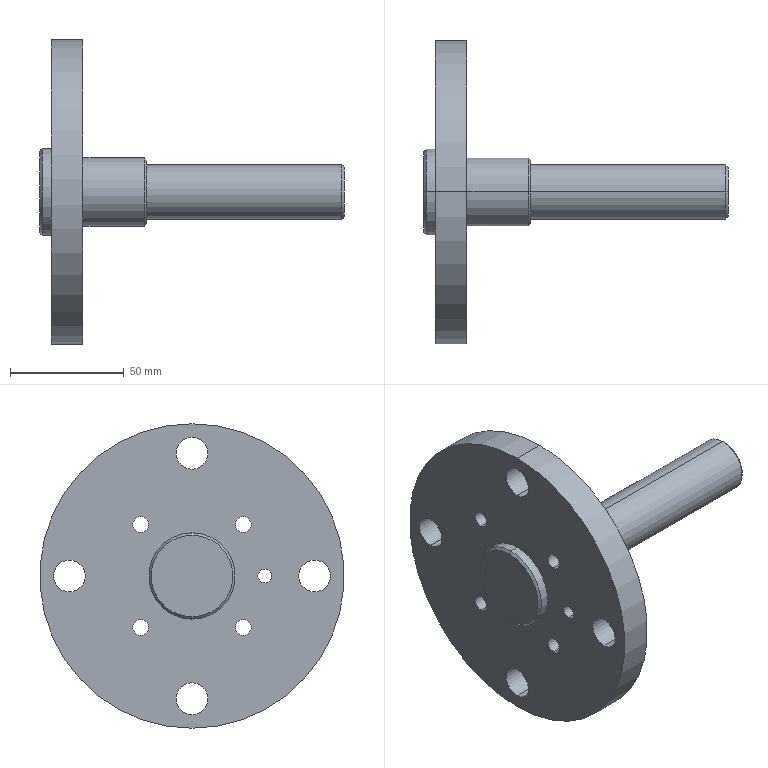Part | SolidWorks | features ICE 8, Chamfer 2, CirPattern 2, Revolution 1 | 1 solid | 49 faces | box 134 x 134 x 134 mm | volume 249153 mm3 | cylinder 34 | plane 9 | cone 6 | commonest cylinder face diameters 7 x8 12 x8 14 x8 6 x2 24 x2 30 x2
STEP:
#1=CARTESIAN_POINT('',(92.,0.,47.));
#2=VERTEX_POINT('',#1);
#3=CARTESIAN_POINT('',(92.,0.,61.));
#4=VERTEX_POINT('',#3);
#5=CARTESIAN_POINT('',(92.,0.,54.));
#6=DIRECTION('',(-1.,0.,0.));
#7=DIRECTION('',(0.,0.,1.));
#8=AXIS2_PLACEMENT_3D('',#5,#6,#7);
#9=CIRCLE('',#8,7.);
#10=EDGE_CURVE('',#2,#4,#9,.T.);
#11=ORIENTED_EDGE('',*,*,#10,.F.);
#12=CARTESIAN_POINT('',(78.,0.,47.));
#13=VERTEX_POINT('',#12);
#14=CARTESIAN_POINT('',(119.,0.,47.));
#15=DIRECTION('',(-1.,0.,0.));
#16=VECTOR('',#15,1000.);
#17=LINE('',#14,#16);
#18=EDGE_CURVE('',#2,#13,#17,.T.);
#19=ORIENTED_EDGE('',*,*,#18,.T.);
#20=CARTESIAN_POINT('',(78.,0.,61.));
#21=VERTEX_POINT('',#20);
#22=CARTESIAN_POINT('',(78.,0.,54.));
#23=DIRECTION('',(-1.,0.,0.));
#24=DIRECTION('',(0.,1.,0.));
#25=AXIS2_PLACEMENT_3D('',#22,#23,#24);
#26=CIRCLE('',#25,7.);
#27=EDGE_CURVE('',#13,#21,#26,.T.);
#28=ORIENTED_EDGE('',*,*,#27,.T.);
#29=CARTESIAN_POINT('',(119.,0.,61.));
#30=DIRECTION('',(-1.,0.,0.));
#31=VECTOR('',#30,1000.);
#32=LINE('',#29,#31);
#33=EDGE_CURVE('',#4,#21,#32,.T.);
#34=ORIENTED_EDGE('',*,*,#33,.F.);
#35=EDGE_LOOP('',(#11,#19,#28,#34));
#36=FACE_OUTER_BOUND('',#35,.T.);
#37=CARTESIAN_POINT('',(119.,0.,54.));
#38=DIRECTION('',(-1.,0.,0.));
#39=DIRECTION('',(0.,0.,1.));
#40=AXIS2_PLACEMENT_3D('',#37,#38,#39);
#41=CYLINDRICAL_SURFACE('',#40,7.);
#42=ADVANCED_FACE('',(#36),#41,.F.);
#43=CARTESIAN_POINT('',(92.,54.,-7.));
#44=VERTEX_POINT('',#43);
#45=CARTESIAN_POINT('',(92.,54.,7.));
#46=VERTEX_POINT('',#45);
#47=CARTESIAN_POINT('',(92.,54.,0.));
#48=DIRECTION('',(-1.,0.,0.));
#49=DIRECTION('',(0.,0.,1.));
#50=AXIS2_PLACEMENT_3D('',#47,#48,#49);
#51=CIRCLE('',#50,7.);
#52=EDGE_CURVE('',#44,#46,#51,.T.);
#53=ORIENTED_EDGE('',*,*,#52,.F.);
#54=CARTESIAN_POINT('',(78.,54.,-7.));
#55=VERTEX_POINT('',#54);
#56=CARTESIAN_POINT('',(119.,54.,-7.));
#57=DIRECTION('',(-1.,0.,0.));
#58=VECTOR('',#57,1000.);
#59=LINE('',#56,#58);
#60=EDGE_CURVE('',#44,#55,#59,.T.);
#61=ORIENTED_EDGE('',*,*,#60,.T.);
#62=CARTESIAN_POINT('',(78.,54.,7.));
#63=VERTEX_POINT('',#62);
#64=CARTESIAN_POINT('',(78.,54.,0.));
#65=DIRECTION('',(-1.,0.,0.));
#66=DIRECTION('',(0.,0.,-1.));
#67=AXIS2_PLACEMENT_3D('',#64,#65,#66);
#68=CIRCLE('',#67,7.);
#69=EDGE_CURVE('',#55,#63,#68,.T.);
#70=ORIENTED_EDGE('',*,*,#69,.T.);
#71=CARTESIAN_POINT('',(119.,54.,7.));
#72=DIRECTION('',(-1.,0.,0.));
#73=VECTOR('',#72,1000.);
#74=LINE('',#71,#73);
#75=EDGE_CURVE('',#46,#63,#74,.T.);
#76=ORIENTED_EDGE('',*,*,#75,.F.);
#77=EDGE_LOOP('',(#53,#61,#70,#76));
#78=FACE_OUTER_BOUND('',#77,.T.);
#79=CARTESIAN_POINT('',(119.,54.,0.));
#80=DIRECTION('',(-1.,0.,0.));
#81=DIRECTION('',(0.,0.,1.));
#82=AXIS2_PLACEMENT_3D('',#79,#80,#81);
#83=CYLINDRICAL_SURFACE('',#82,7.);
#84=ADVANCED_FACE('',(#78),#83,.F.);
#85=CARTESIAN_POINT('',(92.,0.,-61.));
#86=VERTEX_POINT('',#85);
#87=CARTESIAN_POINT('',(92.,0.,-47.));
#88=VERTEX_POINT('',#87);
#89=CARTESIAN_POINT('',(92.,0.,-54.));
#90=DIRECTION('',(-1.,0.,0.));
#91=DIRECTION('',(0.,0.,1.));
#92=AXIS2_PLACEMENT_3D('',#89,#90,#91);
#93=CIRCLE('',#92,7.);
#94=EDGE_CURVE('',#86,#88,#93,.T.);
#95=ORIENTED_EDGE('',*,*,#94,.F.);
#96=CARTESIAN_POINT('',(78.,0.,-61.));
#97=VERTEX_POINT('',#96);
#98=CARTESIAN_POINT('',(119.,0.,-61.));
#99=DIRECTION('',(-1.,0.,0.));
#100=VECTOR('',#99,1000.);
#101=LINE('',#98,#100);
#102=EDGE_CURVE('',#86,#97,#101,.T.);
#103=ORIENTED_EDGE('',*,*,#102,.T.);
#104=CARTESIAN_POINT('',(78.,0.,-47.));
#105=VERTEX_POINT('',#104);
#106=CARTESIAN_POINT('',(78.,0.,-54.));
#107=DIRECTION('',(-1.,0.,0.));
#108=DIRECTION('',(0.,-1.,0.));
#109=AXIS2_PLACEMENT_3D('',#106,#107,#108);
#110=CIRCLE('',#109,7.);
#111=EDGE_CURVE('',#97,#105,#110,.T.);
#112=ORIENTED_EDGE('',*,*,#111,.T.);
#113=CARTESIAN_POINT('',(119.,0.,-47.));
#114=DIRECTION('',(-1.,0.,0.));
#115=VECTOR('',#114,1000.);
#116=LINE('',#113,#115);
#117=EDGE_CURVE('',#88,#105,#116,.T.);
#118=ORIENTED_EDGE('',*,*,#117,.F.);
#119=EDGE_LOOP('',(#95,#103,#112,#118));
#120=FACE_OUTER_BOUND('',#119,.T.);
#121=CARTESIAN_POINT('',(119.,0.,-54.));
#122=DIRECTION('',(-1.,0.,0.));
#123=DIRECTION('',(0.,0.,1.));
#124=AXIS2_PLACEMENT_3D('',#121,#122,#123);
#125=CYLINDRICAL_SURFACE('',#124,7.);
#126=ADVANCED_FACE('',(#120),#125,.F.);
#127=CARTESIAN_POINT('',(92.,-54.,-7.));
#128=VERTEX_POINT('',#127);
#129=CARTESIAN_POINT('',(92.,-54.,7.));
#130=VERTEX_POINT('',#129);
#131=CARTESIAN_POINT('',(92.,-54.,0.));
#132=DIRECTION('',(-1.,0.,0.));
#133=DIRECTION('',(0.,0.,1.));
#134=AXIS2_PLACEMENT_3D('',#131,#132,#133);
#135=CIRCLE('',#134,7.);
#136=EDGE_CURVE('',#128,#130,#135,.T.);
#137=ORIENTED_EDGE('',*,*,#136,.F.);
#138=CARTESIAN_POINT('',(78.,-54.,-7.));
#139=VERTEX_POINT('',#138);
#140=CARTESIAN_POINT('',(119.,-54.,-7.));
#141=DIRECTION('',(-1.,0.,0.));
#142=VECTOR('',#141,1000.);
#143=LINE('',#140,#142);
#144=EDGE_CURVE('',#128,#139,#143,.T.);
#145=ORIENTED_EDGE('',*,*,#144,.T.);
#146=CARTESIAN_POINT('',(78.,-54.,7.));
#147=VERTEX_POINT('',#146);
#148=CARTESIAN_POINT('',(78.,-54.,0.));
#149=DIRECTION('',(-1.,0.,0.));
#150=DIRECTION('',(0.,0.,1.));
#151=AXIS2_PLACEMENT_3D('',#148,#149,#150);
#152=CIRCLE('',#151,7.);
#153=EDGE_CURVE('',#139,#147,#152,.T.);
#154=ORIENTED_EDGE('',*,*,#153,.T.);
#155=CARTESIAN_POINT('',(119.,-54.,7.));
#156=DIRECTION('',(-1.,0.,0.));
#157=VECTOR('',#156,1000.);
#158=LINE('',#155,#157);
#159=EDGE_CURVE('',#130,#147,#158,.T.);
#160=ORIENTED_EDGE('',*,*,#159,.F.);
#161=EDGE_LOOP('',(#137,#145,#154,#160));
#162=FACE_OUTER_BOUND('',#161,.T.);
#163=CARTESIAN_POINT('',(119.,-54.,0.));
#164=DIRECTION('',(-1.,0.,0.));
#165=DIRECTION('',(0.,0.,1.));
#166=AXIS2_PLACEMENT_3D('',#163,#164,#165);
#167=CYLINDRICAL_SURFACE('',#166,7.);
#168=ADVANCED_FACE('',(#162),#167,.F.);
#169=CARTESIAN_POINT('',(73.,0.,18.));
#170=VERTEX_POINT('',#169);
#171=CARTESIAN_POINT('',(73.,0.,-18.));
#172=VERTEX_POINT('',#171);
#173=CARTESIAN_POINT('',(73.,0.,0.));
#174=DIRECTION('',(-1.,0.,0.));
#175=DIRECTION('',(0.,0.,1.));
#176=AXIS2_PLACEMENT_3D('',#173,#174,#175);
#177=CIRCLE('',#176,18.);
#178=EDGE_CURVE('',#170,#172,#177,.T.);
#179=ORIENTED_EDGE('',*,*,#178,.F.);
#180=CARTESIAN_POINT('',(74.,0.,19.));
#181=VERTEX_POINT('',#180);
#182=CARTESIAN_POINT('',(73.,0.,18.));
#183=DIRECTION('',(0.7071,0.,0.7071));
#184=VECTOR('',#183,1000.);
#185=LINE('',#182,#184);
#186=EDGE_CURVE('',#170,#181,#185,.T.);
#187=ORIENTED_EDGE('',*,*,#186,.T.);
#188=CARTESIAN_POINT('',(74.,0.,-19.));
#189=VERTEX_POINT('',#188);
#190=CARTESIAN_POINT('',(74.,0.,0.));
#191=DIRECTION('',(1.,0.,0.));
#192=DIRECTION('',(0.,0.,1.));
#193=AXIS2_PLACEMENT_3D('',#190,#191,#192);
#194=CIRCLE('',#193,19.);
#195=EDGE_CURVE('',#189,#181,#194,.T.);
#196=ORIENTED_EDGE('',*,*,#195,.F.);
#197=CARTESIAN_POINT('',(73.,0.,-18.));
#198=DIRECTION('',(0.7071,0.,-0.7071));
#199=VECTOR('',#198,1000.);
#200=LINE('',#197,#199);
#201=EDGE_CURVE('',#172,#189,#200,.T.);
#202=ORIENTED_EDGE('',*,*,#201,.F.);
#203=EDGE_LOOP('',(#179,#187,#196,#202));
#204=FACE_OUTER_BOUND('',#203,.T.);
#205=CARTESIAN_POINT('',(73.,0.,0.));
#206=DIRECTION('',(1.,0.,0.));
#207=DIRECTION('',(0.,0.,-1.));
#208=AXIS2_PLACEMENT_3D('',#205,#206,#207);
#209=CONICAL_SURFACE('',#208,18.,0.7854);
#210=ADVANCED_FACE('',(#204),#209,.T.);
#211=CARTESIAN_POINT('',(86.,22.627,28.627));
#212=VERTEX_POINT('',#211);
#213=CARTESIAN_POINT('',(86.,22.627,16.627));
#214=VERTEX_POINT('',#213);
#215=CARTESIAN_POINT('',(86.,22.627,22.627));
#216=DIRECTION('',(1.,0.,0.));
#217=DIRECTION('',(0.,0.,-1.));
#218=AXIS2_PLACEMENT_3D('',#215,#216,#217);
#219=CIRCLE('',#218,6.);
#220=EDGE_CURVE('',#212,#214,#219,.T.);
#221=ORIENTED_EDGE('',*,*,#220,.F.);
#222=CARTESIAN_POINT('',(92.,22.627,28.627));
#223=VERTEX_POINT('',#222);
#224=CARTESIAN_POINT('',(86.,22.627,28.627));
#225=DIRECTION('',(1.,0.,0.));
#226=VECTOR('',#225,1000.);
#227=LINE('',#224,#226);
#228=EDGE_CURVE('',#212,#223,#227,.T.);
#229=ORIENTED_EDGE('',*,*,#228,.T.);
#230=CARTESIAN_POINT('',(92.,22.627,16.627));
#231=VERTEX_POINT('',#230);
#232=CARTESIAN_POINT('',(92.,22.627,22.627));
#233=DIRECTION('',(1.,0.,0.));
#234=DIRECTION('',(0.,0.,-1.));
#235=AXIS2_PLACEMENT_3D('',#232,#233,#234);
#236=CIRCLE('',#235,6.);
#237=EDGE_CURVE('',#223,#231,#236,.T.);
#238=ORIENTED_EDGE('',*,*,#237,.T.);
#239=CARTESIAN_POINT('',(86.,22.627,16.627));
#240=DIRECTION('',(1.,0.,0.));
#241=VECTOR('',#240,1000.);
#242=LINE('',#239,#241);
#243=EDGE_CURVE('',#214,#231,#242,.T.);
#244=ORIENTED_EDGE('',*,*,#243,.F.);
#245=EDGE_LOOP('',(#221,#229,#238,#244));
#246=FACE_OUTER_BOUND('',#245,.T.);
#247=CARTESIAN_POINT('',(86.,22.627,22.627));
#248=DIRECTION('',(1.,0.,0.));
#249=DIRECTION('',(0.,0.,-1.));
#250=AXIS2_PLACEMENT_3D('',#247,#248,#249);
#251=CYLINDRICAL_SURFACE('',#250,6.);
#252=ADVANCED_FACE('',(#246),#251,.F.);
#253=CARTESIAN_POINT('',(86.,-22.627,28.627));
#254=VERTEX_POINT('',#253);
#255=CARTESIAN_POINT('',(86.,-22.627,16.627));
#256=VERTEX_POINT('',#255);
#257=CARTESIAN_POINT('',(86.,-22.627,22.627));
#258=DIRECTION('',(1.,0.,0.));
#259=DIRECTION('',(0.,0.,-1.));
#260=AXIS2_PLACEMENT_3D('',#257,#258,#259);
#261=CIRCLE('',#260,6.);
#262=EDGE_CURVE('',#254,#256,#261,.T.);
#263=ORIENTED_EDGE('',*,*,#262,.F.);
#264=CARTESIAN_POINT('',(92.,-22.627,28.627));
#265=VERTEX_POINT('',#264);
#266=CARTESIAN_POINT('',(86.,-22.627,28.627));
#267=DIRECTION('',(1.,0.,0.));
#268=VECTOR('',#267,1000.);
#269=LINE('',#266,#268);
#270=EDGE_CURVE('',#254,#265,#269,.T.);
#271=ORIENTED_EDGE('',*,*,#270,.T.);
#272=CARTESIAN_POINT('',(92.,-22.627,16.627));
#273=VERTEX_POINT('',#272);
#274=CARTESIAN_POINT('',(92.,-22.627,22.627));
#275=DIRECTION('',(1.,0.,0.));
#276=DIRECTION('',(0.,0.,-1.));
#277=AXIS2_PLACEMENT_3D('',#274,#275,#276);
#278=CIRCLE('',#277,6.);
#279=EDGE_CURVE('',#265,#273,#278,.T.);
#280=ORIENTED_EDGE('',*,*,#279,.T.);
#281=CARTESIAN_POINT('',(86.,-22.627,16.627));
#282=DIRECTION('',(1.,0.,0.));
#283=VECTOR('',#282,1000.);
#284=LINE('',#281,#283);
#285=EDGE_CURVE('',#256,#273,#284,.T.);
#286=ORIENTED_EDGE('',*,*,#285,.F.);
#287=EDGE_LOOP('',(#263,#271,#280,#286));
#288=FACE_OUTER_BOUND('',#287,.T.);
#289=CARTESIAN_POINT('',(86.,-22.627,22.627));
#290=DIRECTION('',(1.,0.,0.));
#291=DIRECTION('',(0.,0.,-1.));
#292=AXIS2_PLACEMENT_3D('',#289,#290,#291);
#293=CYLINDRICAL_SURFACE('',#292,6.);
#294=ADVANCED_FACE('',(#288),#293,.F.);
#295=CARTESIAN_POINT('',(86.,-22.627,-16.627));
#296=VERTEX_POINT('',#295);
#297=CARTESIAN_POINT('',(86.,-22.627,-28.627));
#298=VERTEX_POINT('',#297);
#299=CARTESIAN_POINT('',(86.,-22.627,-22.627));
#300=DIRECTION('',(1.,0.,0.));
#301=DIRECTION('',(0.,0.,-1.));
#302=AXIS2_PLACEMENT_3D('',#299,#300,#301);
#303=CIRCLE('',#302,6.);
#304=EDGE_CURVE('',#296,#298,#303,.T.);
#305=ORIENTED_EDGE('',*,*,#304,.F.);
#306=CARTESIAN_POINT('',(92.,-22.627,-16.627));
#307=VERTEX_POINT('',#306);
#308=CARTESIAN_POINT('',(86.,-22.627,-16.627));
#309=DIRECTION('',(1.,0.,0.));
#310=VECTOR('',#309,1000.);
#311=LINE('',#308,#310);
#312=EDGE_CURVE('',#296,#307,#311,.T.);
#313=ORIENTED_EDGE('',*,*,#312,.T.);
#314=CARTESIAN_POINT('',(92.,-22.627,-28.627));
#315=VERTEX_POINT('',#314);
#316=CARTESIAN_POINT('',(92.,-22.627,-22.627));
#317=DIRECTION('',(1.,0.,0.));
#318=DIRECTION('',(0.,0.,-1.));
#319=AXIS2_PLACEMENT_3D('',#316,#317,#318);
#320=CIRCLE('',#319,6.);
#321=EDGE_CURVE('',#307,#315,#320,.T.);
#322=ORIENTED_EDGE('',*,*,#321,.T.);
#323=CARTESIAN_POINT('',(86.,-22.627,-28.627));
#324=DIRECTION('',(1.,0.,0.));
#325=VECTOR('',#324,1000.);
#326=LINE('',#323,#325);
#327=EDGE_CURVE('',#298,#315,#326,.T.);
#328=ORIENTED_EDGE('',*,*,#327,.F.);
#329=EDGE_LOOP('',(#305,#313,#322,#328));
#330=FACE_OUTER_BOUND('',#329,.T.);
#331=CARTESIAN_POINT('',(86.,-22.627,-22.627));
#332=DIRECTION('',(1.,0.,0.));
#333=DIRECTION('',(0.,0.,-1.));
#334=AXIS2_PLACEMENT_3D('',#331,#332,#333);
#335=CYLINDRICAL_SURFACE('',#334,6.);
#336=ADVANCED_FACE('',(#330),#335,.F.);
#337=CARTESIAN_POINT('',(86.,22.627,-16.627));
#338=VERTEX_POINT('',#337);
#339=CARTESIAN_POINT('',(86.,22.627,-28.627));
#340=VERTEX_POINT('',#339);
#341=CARTESIAN_POINT('',(86.,22.627,-22.627));
#342=DIRECTION('',(1.,0.,0.));
#343=DIRECTION('',(0.,0.,-1.));
#344=AXIS2_PLACEMENT_3D('',#341,#342,#343);
#345=CIRCLE('',#344,6.);
#346=EDGE_CURVE('',#338,#340,#345,.T.);
#347=ORIENTED_EDGE('',*,*,#346,.F.);
#348=CARTESIAN_POINT('',(92.,22.627,-16.627));
#349=VERTEX_POINT('',#348);
#350=CARTESIAN_POINT('',(86.,22.627,-16.627));
#351=DIRECTION('',(1.,0.,0.));
#352=VECTOR('',#351,1000.);
#353=LINE('',#350,#352);
#354=EDGE_CURVE('',#338,#349,#353,.T.);
#355=ORIENTED_EDGE('',*,*,#354,.T.);
#356=CARTESIAN_POINT('',(92.,22.627,-28.627));
#357=VERTEX_POINT('',#356);
#358=CARTESIAN_POINT('',(92.,22.627,-22.627));
#359=DIRECTION('',(1.,0.,0.));
#360=DIRECTION('',(0.,0.,-1.));
#361=AXIS2_PLACEMENT_3D('',#358,#359,#360);
#362=CIRCLE('',#361,6.);
#363=EDGE_CURVE('',#349,#357,#362,.T.);
#364=ORIENTED_EDGE('',*,*,#363,.T.);
#365=CARTESIAN_POINT('',(86.,22.627,-28.627));
#366=DIRECTION('',(1.,0.,0.));
#367=VECTOR('',#366,1000.);
#368=LINE('',#365,#367);
#369=EDGE_CURVE('',#340,#357,#368,.T.);
#370=ORIENTED_EDGE('',*,*,#369,.F.);
#371=EDGE_LOOP('',(#347,#355,#364,#370));
#372=FACE_OUTER_BOUND('',#371,.T.);
#373=CARTESIAN_POINT('',(86.,22.627,-22.627));
#374=DIRECTION('',(1.,0.,0.));
#375=DIRECTION('',(0.,0.,-1.));
#376=AXIS2_PLACEMENT_3D('',#373,#374,#375);
#377=CYLINDRICAL_SURFACE('',#376,6.);
#378=ADVANCED_FACE('',(#372),#377,.F.);
#379=CARTESIAN_POINT('',(92.,-32.,-3.));
#380=VERTEX_POINT('',#379);
#381=CARTESIAN_POINT('',(92.,-32.,3.));
#382=VERTEX_POINT('',#381);
#383=CARTESIAN_POINT('',(92.,-32.,0.));
#384=DIRECTION('',(-1.,0.,0.));
#385=DIRECTION('',(0.,0.,1.));
#386=AXIS2_PLACEMENT_3D('',#383,#384,#385);
#387=CIRCLE('',#386,3.);
#388=EDGE_CURVE('',#380,#382,#387,.T.);
#389=ORIENTED_EDGE('',*,*,#388,.F.);
#390=CARTESIAN_POINT('',(78.,-32.,-3.));
#391=VERTEX_POINT('',#390);
#392=CARTESIAN_POINT('',(119.,-32.,-3.));
#393=DIRECTION('',(-1.,0.,0.));
#394=VECTOR('',#393,1000.);
#395=LINE('',#392,#394);
#396=EDGE_CURVE('',#380,#391,#395,.T.);
#397=ORIENTED_EDGE('',*,*,#396,.T.);
#398=CARTESIAN_POINT('',(78.,-32.,3.));
#399=VERTEX_POINT('',#398);
#400=CARTESIAN_POINT('',(78.,-32.,0.));
#401=DIRECTION('',(-1.,0.,0.));
#402=DIRECTION('',(0.,0.,1.));
#403=AXIS2_PLACEMENT_3D('',#400,#401,#402);
#404=CIRCLE('',#403,3.);
#405=EDGE_CURVE('',#391,#399,#404,.T.);
#406=ORIENTED_EDGE('',*,*,#405,.T.);
#407=CARTESIAN_POINT('',(119.,-32.,3.));
#408=DIRECTION('',(-1.,0.,0.));
#409=VECTOR('',#408,1000.);
#410=LINE('',#407,#409);
#411=EDGE_CURVE('',#382,#399,#410,.T.);
#412=ORIENTED_EDGE('',*,*,#411,.F.);
#413=EDGE_LOOP('',(#389,#397,#406,#412));
#414=FACE_OUTER_BOUND('',#413,.T.);
#415=CARTESIAN_POINT('',(119.,-32.,0.));
#416=DIRECTION('',(-1.,0.,0.));
#417=DIRECTION('',(0.,0.,1.));
#418=AXIS2_PLACEMENT_3D('',#415,#416,#417);
#419=CYLINDRICAL_SURFACE('',#418,3.);
#420=ADVANCED_FACE('',(#414),#419,.F.);
#421=ORIENTED_EDGE('',*,*,#195,.T.);
#422=CARTESIAN_POINT('',(78.,0.,19.));
#423=VERTEX_POINT('',#422);
#424=CARTESIAN_POINT('',(73.,0.,19.));
#425=DIRECTION('',(1.,0.,0.));
#426=VECTOR('',#425,1000.);
#427=LINE('',#424,#426);
#428=EDGE_CURVE('',#181,#423,#427,.T.);
#429=ORIENTED_EDGE('',*,*,#428,.T.);
#430=CARTESIAN_POINT('',(78.,0.,-19.));
#431=VERTEX_POINT('',#430);
#432=CARTESIAN_POINT('',(78.,0.,0.));
#433=DIRECTION('',(-1.,0.,0.));
#434=DIRECTION('',(0.,0.,1.));
#435=AXIS2_PLACEMENT_3D('',#432,#433,#434);
#436=CIRCLE('',#435,19.);
#437=EDGE_CURVE('',#423,#431,#436,.T.);
#438=ORIENTED_EDGE('',*,*,#437,.T.);
#439=CARTESIAN_POINT('',(73.,0.,-19.));
#440=DIRECTION('',(1.,0.,0.));
#441=VECTOR('',#440,1000.);
#442=LINE('',#439,#441);
#443=EDGE_CURVE('',#189,#431,#442,.T.);
#444=ORIENTED_EDGE('',*,*,#443,.F.);
#445=EDGE_LOOP('',(#421,#429,#438,#444));
#446=FACE_OUTER_BOUND('',#445,.T.);
#447=CARTESIAN_POINT('',(73.,0.,0.));
#448=DIRECTION('',(1.,0.,0.));
#449=DIRECTION('',(0.,0.,-1.));
#450=AXIS2_PLACEMENT_3D('',#447,#448,#449);
#451=CYLINDRICAL_SURFACE('',#450,19.);
#452=ADVANCED_FACE('',(#446),#451,.T.);
#453=CARTESIAN_POINT('',(78.,0.,67.));
#454=VERTEX_POINT('',#453);
#455=CARTESIAN_POINT('',(78.,0.,-67.));
#456=VERTEX_POINT('',#455);
#457=CARTESIAN_POINT('',(78.,0.,0.));
#458=DIRECTION('',(-1.,0.,0.));
#459=DIRECTION('',(0.,0.,1.));
#460=AXIS2_PLACEMENT_3D('',#457,#458,#459);
#461=CIRCLE('',#460,67.);
#462=EDGE_CURVE('',#454,#456,#461,.T.);
#463=ORIENTED_EDGE('',*,*,#462,.F.);
#464=CARTESIAN_POINT('',(92.,0.,67.));
#465=VERTEX_POINT('',#464);
#466=CARTESIAN_POINT('',(78.,0.,67.));
#467=DIRECTION('',(1.,0.,0.));
#468=VECTOR('',#467,1000.);
#469=LINE('',#466,#468);
#470=EDGE_CURVE('',#454,#465,#469,.T.);
#471=ORIENTED_EDGE('',*,*,#470,.T.);
#472=CARTESIAN_POINT('',(92.,0.,-67.));
#473=VERTEX_POINT('',#472);
#474=CARTESIAN_POINT('',(92.,0.,0.));
#475=DIRECTION('',(-1.,0.,0.));
#476=DIRECTION('',(0.,0.,1.));
#477=AXIS2_PLACEMENT_3D('',#474,#475,#476);
#478=CIRCLE('',#477,67.);
#479=EDGE_CURVE('',#465,#473,#478,.T.);
#480=ORIENTED_EDGE('',*,*,#479,.T.);
#481=CARTESIAN_POINT('',(78.,0.,-67.));
#482=DIRECTION('',(1.,0.,0.));
#483=VECTOR('',#482,1000.);
#484=LINE('',#481,#483);
#485=EDGE_CURVE('',#456,#473,#484,.T.);
#486=ORIENTED_EDGE('',*,*,#485,.F.);
#487=EDGE_LOOP('',(#463,#471,#480,#486));
#488=FACE_OUTER_BOUND('',#487,.T.);
#489=CARTESIAN_POINT('',(78.,0.,0.));
#490=DIRECTION('',(1.,0.,0.));
#491=DIRECTION('',(0.,0.,-1.));
#492=AXIS2_PLACEMENT_3D('',#489,#490,#491);
#493=CYLINDRICAL_SURFACE('',#492,67.);
#494=ADVANCED_FACE('',(#488),#493,.T.);
#495=CARTESIAN_POINT('',(120.,0.,-14.));
#496=VERTEX_POINT('',#495);
#497=CARTESIAN_POINT('',(120.,0.,14.));
#498=VERTEX_POINT('',#497);
#499=CARTESIAN_POINT('',(120.,0.,0.));
#500=DIRECTION('',(1.,0.,0.));
#501=DIRECTION('',(0.,0.,1.));
#502=AXIS2_PLACEMENT_3D('',#499,#500,#501);
#503=CIRCLE('',#502,14.);
#504=EDGE_CURVE('',#496,#498,#503,.T.);
#505=ORIENTED_EDGE('',*,*,#504,.F.);
#506=CARTESIAN_POINT('',(119.,0.,-15.));
#507=VERTEX_POINT('',#506);
#508=CARTESIAN_POINT('',(119.,0.,-15.));
#509=DIRECTION('',(-0.7071,0.,-0.7071));
#510=VECTOR('',#509,1000.);
#511=LINE('',#508,#510);
#512=EDGE_CURVE('',#496,#507,#511,.T.);
#513=ORIENTED_EDGE('',*,*,#512,.T.);
#514=CARTESIAN_POINT('',(119.,0.,15.));
#515=VERTEX_POINT('',#514);
#516=CARTESIAN_POINT('',(119.,0.,0.));
#517=DIRECTION('',(-1.,0.,0.));
#518=DIRECTION('',(0.,0.,1.));
#519=AXIS2_PLACEMENT_3D('',#516,#517,#518);
#520=CIRCLE('',#519,15.);
#521=EDGE_CURVE('',#515,#507,#520,.T.);
#522=ORIENTED_EDGE('',*,*,#521,.F.);
#523=CARTESIAN_POINT('',(119.,0.,15.));
#524=DIRECTION('',(-0.7071,0.,0.7071));
#525=VECTOR('',#524,1000.);
#526=LINE('',#523,#525);
#527=EDGE_CURVE('',#498,#515,#526,.T.);
#528=ORIENTED_EDGE('',*,*,#527,.F.);
#529=EDGE_LOOP('',(#505,#513,#522,#528));
#530=FACE_OUTER_BOUND('',#529,.T.);
#531=CARTESIAN_POINT('',(119.,0.,0.));
#532=DIRECTION('',(-1.,0.,0.));
#533=DIRECTION('',(0.,0.,1.));
#534=AXIS2_PLACEMENT_3D('',#531,#532,#533);
#535=CONICAL_SURFACE('',#534,15.,0.7854);
#536=ADVANCED_FACE('',(#530),#535,.T.);
#537=CARTESIAN_POINT('',(207.,0.,-11.));
#538=VERTEX_POINT('',#537);
#539=CARTESIAN_POINT('',(207.,0.,11.));
#540=VERTEX_POINT('',#539);
#541=CARTESIAN_POINT('',(207.,0.,0.));
#542=DIRECTION('',(1.,0.,0.));
#543=DIRECTION('',(0.,0.,1.));
#544=AXIS2_PLACEMENT_3D('',#541,#542,#543);
#545=CIRCLE('',#544,11.);
#546=EDGE_CURVE('',#538,#540,#545,.T.);
#547=ORIENTED_EDGE('',*,*,#546,.F.);
#548=CARTESIAN_POINT('',(206.,0.,-12.));
#549=VERTEX_POINT('',#548);
#550=CARTESIAN_POINT('',(206.,0.,-12.));
#551=DIRECTION('',(-0.7071,0.,-0.7071));
#552=VECTOR('',#551,1000.);
#553=LINE('',#550,#552);
#554=EDGE_CURVE('',#538,#549,#553,.T.);
#555=ORIENTED_EDGE('',*,*,#554,.T.);
#556=CARTESIAN_POINT('',(206.,0.,12.));
#557=VERTEX_POINT('',#556);
#558=CARTESIAN_POINT('',(206.,0.,0.));
#559=DIRECTION('',(-1.,0.,0.));
#560=DIRECTION('',(0.,0.,1.));
#561=AXIS2_PLACEMENT_3D('',#558,#559,#560);
#562=CIRCLE('',#561,12.);
#563=EDGE_CURVE('',#557,#549,#562,.T.);
#564=ORIENTED_EDGE('',*,*,#563,.F.);
#565=CARTESIAN_POINT('',(206.,0.,12.));
#566=DIRECTION('',(-0.7071,0.,0.7071));
#567=VECTOR('',#566,1000.);
#568=LINE('',#565,#567);
#569=EDGE_CURVE('',#540,#557,#568,.T.);
#570=ORIENTED_EDGE('',*,*,#569,.F.);
#571=EDGE_LOOP('',(#547,#555,#564,#570));
#572=FACE_OUTER_BOUND('',#571,.T.);
#573=CARTESIAN_POINT('',(206.,0.,0.));
#574=DIRECTION('',(-1.,0.,0.));
#575=DIRECTION('',(0.,0.,1.));
#576=AXIS2_PLACEMENT_3D('',#573,#574,#575);
#577=CONICAL_SURFACE('',#576,12.,0.7854);
#578=ADVANCED_FACE('',(#572),#577,.T.);
#579=ORIENTED_EDGE('',*,*,#563,.T.);
#580=CARTESIAN_POINT('',(120.,0.,-12.));
#581=VERTEX_POINT('',#580);
#582=CARTESIAN_POINT('',(0.,0.,-12.));
#583=DIRECTION('',(-1.,0.,0.));
#584=VECTOR('',#583,1000.);
#585=LINE('',#582,#584);
#586=EDGE_CURVE('',#549,#581,#585,.T.);
#587=ORIENTED_EDGE('',*,*,#586,.T.);
#588=CARTESIAN_POINT('',(120.,0.,12.));
#589=VERTEX_POINT('',#588);
#590=CARTESIAN_POINT('',(120.,0.,0.));
#591=DIRECTION('',(-1.,0.,0.));
#592=DIRECTION('',(0.,0.,1.));
#593=AXIS2_PLACEMENT_3D('',#590,#591,#592);
#594=CIRCLE('',#593,12.);
#595=EDGE_CURVE('',#589,#581,#594,.T.);
#596=ORIENTED_EDGE('',*,*,#595,.F.);
#597=CARTESIAN_POINT('',(0.,0.,12.));
#598=DIRECTION('',(-1.,0.,0.));
#599=VECTOR('',#598,1000.);
#600=LINE('',#597,#599);
#601=EDGE_CURVE('',#557,#589,#600,.T.);
#602=ORIENTED_EDGE('',*,*,#601,.F.);
#603=EDGE_LOOP('',(#579,#587,#596,#602));
#604=FACE_OUTER_BOUND('',#603,.T.);
#605=CARTESIAN_POINT('',(0.,0.,0.));
#606=DIRECTION('',(-1.,0.,0.));
#607=DIRECTION('',(0.,0.,1.));
#608=AXIS2_PLACEMENT_3D('',#605,#606,#607);
#609=CYLINDRICAL_SURFACE('',#608,12.);
#610=ADVANCED_FACE('',(#604),#609,.T.);
#611=ORIENTED_EDGE('',*,*,#521,.T.);
#612=CARTESIAN_POINT('',(92.,0.,-15.));
#613=VERTEX_POINT('',#612);
#614=CARTESIAN_POINT('',(0.,0.,-15.));
#615=DIRECTION('',(-1.,0.,0.));
#616=VECTOR('',#615,1000.);
#617=LINE('',#614,#616);
#618=EDGE_CURVE('',#507,#613,#617,.T.);
#619=ORIENTED_EDGE('',*,*,#618,.T.);
#620=CARTESIAN_POINT('',(92.,0.,15.));
#621=VERTEX_POINT('',#620);
#622=CARTESIAN_POINT('',(92.,0.,0.));
#623=DIRECTION('',(-1.,0.,0.));
#624=DIRECTION('',(0.,0.,1.));
#625=AXIS2_PLACEMENT_3D('',#622,#623,#624);
#626=CIRCLE('',#625,15.);
#627=EDGE_CURVE('',#621,#613,#626,.T.);
#628=ORIENTED_EDGE('',*,*,#627,.F.);
#629=CARTESIAN_POINT('',(0.,0.,15.));
#630=DIRECTION('',(-1.,0.,0.));
#631=VECTOR('',#630,1000.);
#632=LINE('',#629,#631);
#633=EDGE_CURVE('',#515,#621,#632,.T.);
#634=ORIENTED_EDGE('',*,*,#633,.F.);
#635=EDGE_LOOP('',(#611,#619,#628,#634));
#636=FACE_OUTER_BOUND('',#635,.T.);
#637=CARTESIAN_POINT('',(0.,0.,0.));
#638=DIRECTION('',(-1.,0.,0.));
#639=DIRECTION('',(0.,0.,1.));
#640=AXIS2_PLACEMENT_3D('',#637,#638,#639);
#641=CYLINDRICAL_SURFACE('',#640,15.);
#642=ADVANCED_FACE('',(#636),#641,.T.);
#643=CARTESIAN_POINT('',(86.,22.627,-26.127));
#644=VERTEX_POINT('',#643);
#645=CARTESIAN_POINT('',(86.,22.627,-19.127));
#646=VERTEX_POINT('',#645);
#647=CARTESIAN_POINT('',(86.,22.627,-22.627));
#648=DIRECTION('',(-1.,0.,0.));
#649=DIRECTION('',(0.,0.,-1.));
#650=AXIS2_PLACEMENT_3D('',#647,#648,#649);
#651=CIRCLE('',#650,3.5);
#652=EDGE_CURVE('',#644,#646,#651,.T.);
#653=ORIENTED_EDGE('',*,*,#652,.F.);
#654=CARTESIAN_POINT('',(78.,22.627,-26.127));
#655=VERTEX_POINT('',#654);
#656=CARTESIAN_POINT('',(119.,22.627,-26.127));
#657=DIRECTION('',(-1.,0.,0.));
#658=VECTOR('',#657,1000.);
#659=LINE('',#656,#658);
#660=EDGE_CURVE('',#644,#655,#659,.T.);
#661=ORIENTED_EDGE('',*,*,#660,.T.);
#662=CARTESIAN_POINT('',(78.,22.627,-19.127));
#663=VERTEX_POINT('',#662);
#664=CARTESIAN_POINT('',(78.,22.627,-22.627));
#665=DIRECTION('',(-1.,0.,0.));
#666=DIRECTION('',(0.,0.,1.));
#667=AXIS2_PLACEMENT_3D('',#664,#665,#666);
#668=CIRCLE('',#667,3.5);
#669=EDGE_CURVE('',#655,#663,#668,.T.);
#670=ORIENTED_EDGE('',*,*,#669,.T.);
#671=CARTESIAN_POINT('',(119.,22.627,-19.127));
#672=DIRECTION('',(-1.,0.,0.));
#673=VECTOR('',#672,1000.);
#674=LINE('',#671,#673);
#675=EDGE_CURVE('',#646,#663,#674,.T.);
#676=ORIENTED_EDGE('',*,*,#675,.F.);
#677=EDGE_LOOP('',(#653,#661,#670,#676));
#678=FACE_OUTER_BOUND('',#677,.T.);
#679=CARTESIAN_POINT('',(119.,22.627,-22.627));
#680=DIRECTION('',(-1.,0.,0.));
#681=DIRECTION('',(0.,0.,1.));
#682=AXIS2_PLACEMENT_3D('',#679,#680,#681);
#683=CYLINDRICAL_SURFACE('',#682,3.5);
#684=ADVANCED_FACE('',(#678),#683,.F.);
#685=CARTESIAN_POINT('',(86.,-22.627,-26.127));
#686=VERTEX_POINT('',#685);
#687=CARTESIAN_POINT('',(86.,-22.627,-19.127));
#688=VERTEX_POINT('',#687);
#689=CARTESIAN_POINT('',(86.,-22.627,-22.627));
#690=DIRECTION('',(-1.,0.,0.));
#691=DIRECTION('',(0.,0.,-1.));
#692=AXIS2_PLACEMENT_3D('',#689,#690,#691);
#693=CIRCLE('',#692,3.5);
#694=EDGE_CURVE('',#686,#688,#693,.T.);
#695=ORIENTED_EDGE('',*,*,#694,.F.);
#696=CARTESIAN_POINT('',(78.,-22.627,-26.127));
#697=VERTEX_POINT('',#696);
#698=CARTESIAN_POINT('',(119.,-22.627,-26.127));
#699=DIRECTION('',(-1.,0.,0.));
#700=VECTOR('',#699,1000.);
#701=LINE('',#698,#700);
#702=EDGE_CURVE('',#686,#697,#701,.T.);
#703=ORIENTED_EDGE('',*,*,#702,.T.);
#704=CARTESIAN_POINT('',(78.,-22.627,-19.127));
#705=VERTEX_POINT('',#704);
#706=CARTESIAN_POINT('',(78.,-22.627,-22.627));
#707=DIRECTION('',(-1.,0.,0.));
#708=DIRECTION('',(0.,0.,1.));
#709=AXIS2_PLACEMENT_3D('',#706,#707,#708);
#710=CIRCLE('',#709,3.5);
#711=EDGE_CURVE('',#697,#705,#710,.T.);
#712=ORIENTED_EDGE('',*,*,#711,.T.);
#713=CARTESIAN_POINT('',(119.,-22.627,-19.127));
#714=DIRECTION('',(-1.,0.,0.));
#715=VECTOR('',#714,1000.);
#716=LINE('',#713,#715);
#717=EDGE_CURVE('',#688,#705,#716,.T.);
#718=ORIENTED_EDGE('',*,*,#717,.F.);
#719=EDGE_LOOP('',(#695,#703,#712,#718));
#720=FACE_OUTER_BOUND('',#719,.T.);
#721=CARTESIAN_POINT('',(119.,-22.627,-22.627));
#722=DIRECTION('',(-1.,0.,0.));
#723=DIRECTION('',(0.,0.,1.));
#724=AXIS2_PLACEMENT_3D('',#721,#722,#723);
#725=CYLINDRICAL_SURFACE('',#724,3.5);
#726=ADVANCED_FACE('',(#720),#725,.F.);
#727=CARTESIAN_POINT('',(86.,-22.627,19.127));
#728=VERTEX_POINT('',#727);
#729=CARTESIAN_POINT('',(86.,-22.627,26.127));
#730=VERTEX_POINT('',#729);
#731=CARTESIAN_POINT('',(86.,-22.627,22.627));
#732=DIRECTION('',(-1.,0.,0.));
#733=DIRECTION('',(0.,0.,-1.));
#734=AXIS2_PLACEMENT_3D('',#731,#732,#733);
#735=CIRCLE('',#734,3.5);
#736=EDGE_CURVE('',#728,#730,#735,.T.);
#737=ORIENTED_EDGE('',*,*,#736,.F.);
#738=CARTESIAN_POINT('',(78.,-22.627,19.127));
#739=VERTEX_POINT('',#738);
#740=CARTESIAN_POINT('',(119.,-22.627,19.127));
#741=DIRECTION('',(-1.,0.,0.));
#742=VECTOR('',#741,1000.);
#743=LINE('',#740,#742);
#744=EDGE_CURVE('',#728,#739,#743,.T.);
#745=ORIENTED_EDGE('',*,*,#744,.T.);
#746=CARTESIAN_POINT('',(78.,-22.627,26.127));
#747=VERTEX_POINT('',#746);
#748=CARTESIAN_POINT('',(78.,-22.627,22.627));
#749=DIRECTION('',(-1.,0.,0.));
#750=DIRECTION('',(0.,0.,1.));
#751=AXIS2_PLACEMENT_3D('',#748,#749,#750);
#752=CIRCLE('',#751,3.5);
#753=EDGE_CURVE('',#739,#747,#752,.T.);
#754=ORIENTED_EDGE('',*,*,#753,.T.);
#755=CARTESIAN_POINT('',(119.,-22.627,26.127));
#756=DIRECTION('',(-1.,0.,0.));
#757=VECTOR('',#756,1000.);
#758=LINE('',#755,#757);
#759=EDGE_CURVE('',#730,#747,#758,.T.);
#760=ORIENTED_EDGE('',*,*,#759,.F.);
#761=EDGE_LOOP('',(#737,#745,#754,#760));
#762=FACE_OUTER_BOUND('',#761,.T.);
#763=CARTESIAN_POINT('',(119.,-22.627,22.627));
#764=DIRECTION('',(-1.,0.,0.));
#765=DIRECTION('',(0.,0.,1.));
#766=AXIS2_PLACEMENT_3D('',#763,#764,#765);
#767=CYLINDRICAL_SURFACE('',#766,3.5);
#768=ADVANCED_FACE('',(#762),#767,.F.);
#769=CARTESIAN_POINT('',(86.,22.627,19.127));
#770=VERTEX_POINT('',#769);
#771=CARTESIAN_POINT('',(86.,22.627,26.127));
#772=VERTEX_POINT('',#771);
#773=CARTESIAN_POINT('',(86.,22.627,22.627));
#774=DIRECTION('',(-1.,0.,0.));
#775=DIRECTION('',(0.,0.,-1.));
#776=AXIS2_PLACEMENT_3D('',#773,#774,#775);
#777=CIRCLE('',#776,3.5);
#778=EDGE_CURVE('',#770,#772,#777,.T.);
#779=ORIENTED_EDGE('',*,*,#778,.F.);
#780=CARTESIAN_POINT('',(78.,22.627,19.127));
#781=VERTEX_POINT('',#780);
#782=CARTESIAN_POINT('',(119.,22.627,19.127));
#783=DIRECTION('',(-1.,0.,0.));
#784=VECTOR('',#783,1000.);
#785=LINE('',#782,#784);
#786=EDGE_CURVE('',#770,#781,#785,.T.);
#787=ORIENTED_EDGE('',*,*,#786,.T.);
#788=CARTESIAN_POINT('',(78.,22.627,26.127));
#789=VERTEX_POINT('',#788);
#790=CARTESIAN_POINT('',(78.,22.627,22.627));
#791=DIRECTION('',(-1.,0.,0.));
#792=DIRECTION('',(0.,0.,1.));
#793=AXIS2_PLACEMENT_3D('',#790,#791,#792);
#794=CIRCLE('',#793,3.5);
#795=EDGE_CURVE('',#781,#789,#794,.T.);
#796=ORIENTED_EDGE('',*,*,#795,.T.);
#797=CARTESIAN_POINT('',(119.,22.627,26.127));
#798=DIRECTION('',(-1.,0.,0.));
#799=VECTOR('',#798,1000.);
#800=LINE('',#797,#799);
#801=EDGE_CURVE('',#772,#789,#800,.T.);
#802=ORIENTED_EDGE('',*,*,#801,.F.);
#803=EDGE_LOOP('',(#779,#787,#796,#802));
#804=FACE_OUTER_BOUND('',#803,.T.);
#805=CARTESIAN_POINT('',(119.,22.627,22.627));
#806=DIRECTION('',(-1.,0.,0.));
#807=DIRECTION('',(0.,0.,1.));
#808=AXIS2_PLACEMENT_3D('',#805,#806,#807);
#809=CYLINDRICAL_SURFACE('',#808,3.5);
#810=ADVANCED_FACE('',(#804),#809,.F.);
#811=ORIENTED_EDGE('',*,*,#786,.F.);
#812=CARTESIAN_POINT('',(86.,22.627,22.627));
#813=DIRECTION('',(-1.,0.,0.));
#814=DIRECTION('',(0.,0.,-1.));
#815=AXIS2_PLACEMENT_3D('',#812,#813,#814);
#816=CIRCLE('',#815,3.5);
#817=EDGE_CURVE('',#772,#770,#816,.T.);
#818=ORIENTED_EDGE('',*,*,#817,.F.);
#819=ORIENTED_EDGE('',*,*,#801,.T.);
#820=CARTESIAN_POINT('',(78.,22.627,22.627));
#821=DIRECTION('',(-1.,0.,0.));
#822=DIRECTION('',(0.,0.,1.));
#823=AXIS2_PLACEMENT_3D('',#820,#821,#822);
#824=CIRCLE('',#823,3.5);
#825=EDGE_CURVE('',#789,#781,#824,.T.);
#826=ORIENTED_EDGE('',*,*,#825,.T.);
#827=EDGE_LOOP('',(#811,#818,#819,#826));
#828=FACE_OUTER_BOUND('',#827,.T.);
#829=CARTESIAN_POINT('',(119.,22.627,22.627));
#830=DIRECTION('',(-1.,0.,0.));
#831=DIRECTION('',(0.,0.,1.));
#832=AXIS2_PLACEMENT_3D('',#829,#830,#831);
#833=CYLINDRICAL_SURFACE('',#832,3.5);
#834=ADVANCED_FACE('',(#828),#833,.F.);
#835=ORIENTED_EDGE('',*,*,#744,.F.);
#836=CARTESIAN_POINT('',(86.,-22.627,22.627));
#837=DIRECTION('',(-1.,0.,0.));
#838=DIRECTION('',(0.,0.,-1.));
#839=AXIS2_PLACEMENT_3D('',#836,#837,#838);
#840=CIRCLE('',#839,3.5);
#841=EDGE_CURVE('',#730,#728,#840,.T.);
#842=ORIENTED_EDGE('',*,*,#841,.F.);
#843=ORIENTED_EDGE('',*,*,#759,.T.);
#844=CARTESIAN_POINT('',(78.,-22.627,22.627));
#845=DIRECTION('',(-1.,0.,0.));
#846=DIRECTION('',(0.,0.,1.));
#847=AXIS2_PLACEMENT_3D('',#844,#845,#846);
#848=CIRCLE('',#847,3.5);
#849=EDGE_CURVE('',#747,#739,#848,.T.);
#850=ORIENTED_EDGE('',*,*,#849,.T.);
#851=EDGE_LOOP('',(#835,#842,#843,#850));
#852=FACE_OUTER_BOUND('',#851,.T.);
#853=CARTESIAN_POINT('',(119.,-22.627,22.627));
#854=DIRECTION('',(-1.,0.,0.));
#855=DIRECTION('',(0.,0.,1.));
#856=AXIS2_PLACEMENT_3D('',#853,#854,#855);
#857=CYLINDRICAL_SURFACE('',#856,3.5);
#858=ADVANCED_FACE('',(#852),#857,.F.);
#859=ORIENTED_EDGE('',*,*,#702,.F.);
#860=CARTESIAN_POINT('',(86.,-22.627,-22.627));
#861=DIRECTION('',(-1.,0.,0.));
#862=DIRECTION('',(0.,0.,-1.));
#863=AXIS2_PLACEMENT_3D('',#860,#861,#862);
#864=CIRCLE('',#863,3.5);
#865=EDGE_CURVE('',#688,#686,#864,.T.);
#866=ORIENTED_EDGE('',*,*,#865,.F.);
#867=ORIENTED_EDGE('',*,*,#717,.T.);
#868=CARTESIAN_POINT('',(78.,-22.627,-22.627));
#869=DIRECTION('',(-1.,0.,0.));
#870=DIRECTION('',(0.,0.,1.));
#871=AXIS2_PLACEMENT_3D('',#868,#869,#870);
#872=CIRCLE('',#871,3.5);
#873=EDGE_CURVE('',#705,#697,#872,.T.);
#874=ORIENTED_EDGE('',*,*,#873,.T.);
#875=EDGE_LOOP('',(#859,#866,#867,#874));
#876=FACE_OUTER_BOUND('',#875,.T.);
#877=CARTESIAN_POINT('',(119.,-22.627,-22.627));
#878=DIRECTION('',(-1.,0.,0.));
#879=DIRECTION('',(0.,0.,1.));
#880=AXIS2_PLACEMENT_3D('',#877,#878,#879);
#881=CYLINDRICAL_SURFACE('',#880,3.5);
#882=ADVANCED_FACE('',(#876),#881,.F.);
#883=ORIENTED_EDGE('',*,*,#660,.F.);
#884=CARTESIAN_POINT('',(86.,22.627,-22.627));
#885=DIRECTION('',(-1.,0.,0.));
#886=DIRECTION('',(0.,0.,-1.));
#887=AXIS2_PLACEMENT_3D('',#884,#885,#886);
#888=CIRCLE('',#887,3.5);
#889=EDGE_CURVE('',#646,#644,#888,.T.);
#890=ORIENTED_EDGE('',*,*,#889,.F.);
#891=ORIENTED_EDGE('',*,*,#675,.T.);
#892=CARTESIAN_POINT('',(78.,22.627,-22.627));
#893=DIRECTION('',(-1.,0.,0.));
#894=DIRECTION('',(0.,0.,1.));
#895=AXIS2_PLACEMENT_3D('',#892,#893,#894);
#896=CIRCLE('',#895,3.5);
#897=EDGE_CURVE('',#663,#655,#896,.T.);
#898=ORIENTED_EDGE('',*,*,#897,.T.);
#899=EDGE_LOOP('',(#883,#890,#891,#898));
#900=FACE_OUTER_BOUND('',#899,.T.);
#901=CARTESIAN_POINT('',(119.,22.627,-22.627));
#902=DIRECTION('',(-1.,0.,0.));
#903=DIRECTION('',(0.,0.,1.));
#904=AXIS2_PLACEMENT_3D('',#901,#902,#903);
#905=CYLINDRICAL_SURFACE('',#904,3.5);
#906=ADVANCED_FACE('',(#900),#905,.F.);
#907=CARTESIAN_POINT('',(78.,0.,54.));
#908=DIRECTION('',(-1.,0.,0.));
#909=DIRECTION('',(0.,1.,0.));
#910=AXIS2_PLACEMENT_3D('',#907,#908,#909);
#911=CIRCLE('',#910,7.);
#912=EDGE_CURVE('',#21,#13,#911,.T.);
#913=ORIENTED_EDGE('',*,*,#912,.F.);
#914=ORIENTED_EDGE('',*,*,#27,.F.);
#915=EDGE_LOOP('',(#913,#914));
#916=FACE_BOUND('',#915,.T.);
#917=CARTESIAN_POINT('',(78.,54.,0.));
#918=DIRECTION('',(-1.,0.,0.));
#919=DIRECTION('',(0.,0.,-1.));
#920=AXIS2_PLACEMENT_3D('',#917,#918,#919);
#921=CIRCLE('',#920,7.);
#922=EDGE_CURVE('',#63,#55,#921,.T.);
#923=ORIENTED_EDGE('',*,*,#922,.F.);
#924=ORIENTED_EDGE('',*,*,#69,.F.);
#925=EDGE_LOOP('',(#923,#924));
#926=FACE_BOUND('',#925,.T.);
#927=CARTESIAN_POINT('',(78.,0.,-54.));
#928=DIRECTION('',(-1.,0.,0.));
#929=DIRECTION('',(0.,-1.,0.));
#930=AXIS2_PLACEMENT_3D('',#927,#928,#929);
#931=CIRCLE('',#930,7.);
#932=EDGE_CURVE('',#105,#97,#931,.T.);
#933=ORIENTED_EDGE('',*,*,#932,.F.);
#934=ORIENTED_EDGE('',*,*,#111,.F.);
#935=EDGE_LOOP('',(#933,#934));
#936=FACE_BOUND('',#935,.T.);
#937=CARTESIAN_POINT('',(78.,-54.,0.));
#938=DIRECTION('',(-1.,0.,0.));
#939=DIRECTION('',(0.,0.,1.));
#940=AXIS2_PLACEMENT_3D('',#937,#938,#939);
#941=CIRCLE('',#940,7.);
#942=EDGE_CURVE('',#147,#139,#941,.T.);
#943=ORIENTED_EDGE('',*,*,#942,.F.);
#944=ORIENTED_EDGE('',*,*,#153,.F.);
#945=EDGE_LOOP('',(#943,#944));
#946=FACE_BOUND('',#945,.T.);
#947=ORIENTED_EDGE('',*,*,#897,.F.);
#948=ORIENTED_EDGE('',*,*,#669,.F.);
#949=EDGE_LOOP('',(#947,#948));
#950=FACE_BOUND('',#949,.T.);
#951=ORIENTED_EDGE('',*,*,#873,.F.);
#952=ORIENTED_EDGE('',*,*,#711,.F.);
#953=EDGE_LOOP('',(#951,#952));
#954=FACE_BOUND('',#953,.T.);
#955=ORIENTED_EDGE('',*,*,#849,.F.);
#956=ORIENTED_EDGE('',*,*,#753,.F.);
#957=EDGE_LOOP('',(#955,#956));
#958=FACE_BOUND('',#957,.T.);
#959=ORIENTED_EDGE('',*,*,#825,.F.);
#960=ORIENTED_EDGE('',*,*,#795,.F.);
#961=EDGE_LOOP('',(#959,#960));
#962=FACE_BOUND('',#961,.T.);
#963=CARTESIAN_POINT('',(78.,-32.,0.));
#964=DIRECTION('',(-1.,0.,0.));
#965=DIRECTION('',(0.,0.,1.));
#966=AXIS2_PLACEMENT_3D('',#963,#964,#965);
#967=CIRCLE('',#966,3.);
#968=EDGE_CURVE('',#399,#391,#967,.T.);
#969=ORIENTED_EDGE('',*,*,#968,.F.);
#970=ORIENTED_EDGE('',*,*,#405,.F.);
#971=EDGE_LOOP('',(#969,#970));
#972=FACE_BOUND('',#971,.T.);
#973=CARTESIAN_POINT('',(78.,0.,0.));
#974=DIRECTION('',(-1.,0.,0.));
#975=DIRECTION('',(0.,0.,1.));
#976=AXIS2_PLACEMENT_3D('',#973,#974,#975);
#977=CIRCLE('',#976,67.);
#978=EDGE_CURVE('',#456,#454,#977,.T.);
#979=ORIENTED_EDGE('',*,*,#978,.T.);
#980=ORIENTED_EDGE('',*,*,#462,.T.);
#981=EDGE_LOOP('',(#979,#980));
#982=FACE_OUTER_BOUND('',#981,.T.);
#983=CARTESIAN_POINT('',(78.,0.,0.));
#984=DIRECTION('',(-1.,0.,0.));
#985=DIRECTION('',(0.,0.,1.));
#986=AXIS2_PLACEMENT_3D('',#983,#984,#985);
#987=CIRCLE('',#986,19.);
#988=EDGE_CURVE('',#431,#423,#987,.T.);
#989=ORIENTED_EDGE('',*,*,#988,.F.);
#990=ORIENTED_EDGE('',*,*,#437,.F.);
#991=EDGE_LOOP('',(#989,#990));
#992=FACE_BOUND('',#991,.T.);
#993=CARTESIAN_POINT('',(78.,0.,0.));
#994=DIRECTION('',(-1.,0.,0.));
#995=DIRECTION('',(0.,0.,1.));
#996=AXIS2_PLACEMENT_3D('',#993,#994,#995);
#997=PLANE('',#996);
#998=ADVANCED_FACE('',(#916,#926,#936,#946,#950,#954,#958,#962,#972,#982,#992),#997,.T.);
#999=ORIENTED_EDGE('',*,*,#618,.F.);
#1000=CARTESIAN_POINT('',(119.,0.,0.));
#1001=DIRECTION('',(-1.,0.,0.));
#1002=DIRECTION('',(0.,0.,1.));
#1003=AXIS2_PLACEMENT_3D('',#1000,#1001,#1002);
#1004=CIRCLE('',#1003,15.);
#1005=EDGE_CURVE('',#507,#515,#1004,.T.);
#1006=ORIENTED_EDGE('',*,*,#1005,.T.);
#1007=ORIENTED_EDGE('',*,*,#633,.T.);
#1008=CARTESIAN_POINT('',(92.,0.,0.));
#1009=DIRECTION('',(-1.,0.,0.));
#1010=DIRECTION('',(0.,0.,1.));
#1011=AXIS2_PLACEMENT_3D('',#1008,#1009,#1010);
#1012=CIRCLE('',#1011,15.);
#1013=EDGE_CURVE('',#613,#621,#1012,.T.);
#1014=ORIENTED_EDGE('',*,*,#1013,.F.);
#1015=EDGE_LOOP('',(#999,#1006,#1007,#1014));
#1016=FACE_OUTER_BOUND('',#1015,.T.);
#1017=CARTESIAN_POINT('',(0.,0.,0.));
#1018=DIRECTION('',(-1.,0.,0.));
#1019=DIRECTION('',(0.,0.,1.));
#1020=AXIS2_PLACEMENT_3D('',#1017,#1018,#1019);
#1021=CYLINDRICAL_SURFACE('',#1020,15.);
#1022=ADVANCED_FACE('',(#1016),#1021,.T.);
#1023=CARTESIAN_POINT('',(120.,0.,0.));
#1024=DIRECTION('',(1.,0.,0.));
#1025=DIRECTION('',(0.,0.,1.));
#1026=AXIS2_PLACEMENT_3D('',#1023,#1024,#1025);
#1027=CIRCLE('',#1026,14.);
#1028=EDGE_CURVE('',#498,#496,#1027,.T.);
#1029=ORIENTED_EDGE('',*,*,#1028,.T.);
#1030=ORIENTED_EDGE('',*,*,#504,.T.);
#1031=EDGE_LOOP('',(#1029,#1030));
#1032=FACE_OUTER_BOUND('',#1031,.T.);
#1033=ORIENTED_EDGE('',*,*,#595,.T.);
#1034=CARTESIAN_POINT('',(120.,0.,0.));
#1035=DIRECTION('',(-1.,0.,0.));
#1036=DIRECTION('',(0.,0.,1.));
#1037=AXIS2_PLACEMENT_3D('',#1034,#1035,#1036);
#1038=CIRCLE('',#1037,12.);
#1039=EDGE_CURVE('',#581,#589,#1038,.T.);
#1040=ORIENTED_EDGE('',*,*,#1039,.T.);
#1041=EDGE_LOOP('',(#1033,#1040));
#1042=FACE_BOUND('',#1041,.T.);
#1043=CARTESIAN_POINT('',(120.,15.,0.));
#1044=DIRECTION('',(-1.,0.,0.));
#1045=DIRECTION('',(0.,0.,1.));
#1046=AXIS2_PLACEMENT_3D('',#1043,#1044,#1045);
#1047=PLANE('',#1046);
#1048=ADVANCED_FACE('',(#1032,#1042),#1047,.F.);
#1049=ORIENTED_EDGE('',*,*,#586,.F.);
#1050=CARTESIAN_POINT('',(206.,0.,0.));
#1051=DIRECTION('',(-1.,0.,0.));
#1052=DIRECTION('',(0.,0.,1.));
#1053=AXIS2_PLACEMENT_3D('',#1050,#1051,#1052);
#1054=CIRCLE('',#1053,12.);
#1055=EDGE_CURVE('',#549,#557,#1054,.T.);
#1056=ORIENTED_EDGE('',*,*,#1055,.T.);
#1057=ORIENTED_EDGE('',*,*,#601,.T.);
#1058=ORIENTED_EDGE('',*,*,#1039,.F.);
#1059=EDGE_LOOP('',(#1049,#1056,#1057,#1058));
#1060=FACE_OUTER_BOUND('',#1059,.T.);
#1061=CARTESIAN_POINT('',(0.,0.,0.));
#1062=DIRECTION('',(-1.,0.,0.));
#1063=DIRECTION('',(0.,0.,1.));
#1064=AXIS2_PLACEMENT_3D('',#1061,#1062,#1063);
#1065=CYLINDRICAL_SURFACE('',#1064,12.);
#1066=ADVANCED_FACE('',(#1060),#1065,.T.);
#1067=CARTESIAN_POINT('',(207.,0.,0.));
#1068=DIRECTION('',(1.,0.,0.));
#1069=DIRECTION('',(0.,0.,1.));
#1070=AXIS2_PLACEMENT_3D('',#1067,#1068,#1069);
#1071=CIRCLE('',#1070,11.);
#1072=EDGE_CURVE('',#540,#538,#1071,.T.);
#1073=ORIENTED_EDGE('',*,*,#1072,.T.);
#1074=ORIENTED_EDGE('',*,*,#546,.T.);
#1075=EDGE_LOOP('',(#1073,#1074));
#1076=FACE_OUTER_BOUND('',#1075,.T.);
#1077=CARTESIAN_POINT('',(207.,12.,0.));
#1078=DIRECTION('',(-1.,0.,0.));
#1079=DIRECTION('',(0.,0.,1.));
#1080=AXIS2_PLACEMENT_3D('',#1077,#1078,#1079);
#1081=PLANE('',#1080);
#1082=ADVANCED_FACE('',(#1076),#1081,.F.);
#1083=ORIENTED_EDGE('',*,*,#554,.F.);
#1084=ORIENTED_EDGE('',*,*,#1072,.F.);
#1085=ORIENTED_EDGE('',*,*,#569,.T.);
#1086=ORIENTED_EDGE('',*,*,#1055,.F.);
#1087=EDGE_LOOP('',(#1083,#1084,#1085,#1086));
#1088=FACE_OUTER_BOUND('',#1087,.T.);
#1089=CARTESIAN_POINT('',(206.,0.,0.));
#1090=DIRECTION('',(-1.,0.,0.));
#1091=DIRECTION('',(0.,0.,1.));
#1092=AXIS2_PLACEMENT_3D('',#1089,#1090,#1091);
#1093=CONICAL_SURFACE('',#1092,12.,0.7854);
#1094=ADVANCED_FACE('',(#1088),#1093,.T.);
#1095=ORIENTED_EDGE('',*,*,#512,.F.);
#1096=ORIENTED_EDGE('',*,*,#1028,.F.);
#1097=ORIENTED_EDGE('',*,*,#527,.T.);
#1098=ORIENTED_EDGE('',*,*,#1005,.F.);
#1099=EDGE_LOOP('',(#1095,#1096,#1097,#1098));
#1100=FACE_OUTER_BOUND('',#1099,.T.);
#1101=CARTESIAN_POINT('',(119.,0.,0.));
#1102=DIRECTION('',(-1.,0.,0.));
#1103=DIRECTION('',(0.,0.,1.));
#1104=AXIS2_PLACEMENT_3D('',#1101,#1102,#1103);
#1105=CONICAL_SURFACE('',#1104,15.,0.7854);
#1106=ADVANCED_FACE('',(#1100),#1105,.T.);
#1107=CARTESIAN_POINT('',(92.,0.,54.));
#1108=DIRECTION('',(-1.,0.,0.));
#1109=DIRECTION('',(0.,0.,1.));
#1110=AXIS2_PLACEMENT_3D('',#1107,#1108,#1109);
#1111=CIRCLE('',#1110,7.);
#1112=EDGE_CURVE('',#4,#2,#1111,.T.);
#1113=ORIENTED_EDGE('',*,*,#1112,.T.);
#1114=ORIENTED_EDGE('',*,*,#10,.T.);
#1115=EDGE_LOOP('',(#1113,#1114));
#1116=FACE_BOUND('',#1115,.T.);
#1117=CARTESIAN_POINT('',(92.,54.,0.));
#1118=DIRECTION('',(-1.,0.,0.));
#1119=DIRECTION('',(0.,0.,1.));
#1120=AXIS2_PLACEMENT_3D('',#1117,#1118,#1119);
#1121=CIRCLE('',#1120,7.);
#1122=EDGE_CURVE('',#46,#44,#1121,.T.);
#1123=ORIENTED_EDGE('',*,*,#1122,.T.);
#1124=ORIENTED_EDGE('',*,*,#52,.T.);
#1125=EDGE_LOOP('',(#1123,#1124));
#1126=FACE_BOUND('',#1125,.T.);
#1127=CARTESIAN_POINT('',(92.,0.,-54.));
#1128=DIRECTION('',(-1.,0.,0.));
#1129=DIRECTION('',(0.,0.,1.));
#1130=AXIS2_PLACEMENT_3D('',#1127,#1128,#1129);
#1131=CIRCLE('',#1130,7.);
#1132=EDGE_CURVE('',#88,#86,#1131,.T.);
#1133=ORIENTED_EDGE('',*,*,#1132,.T.);
#1134=ORIENTED_EDGE('',*,*,#94,.T.);
#1135=EDGE_LOOP('',(#1133,#1134));
#1136=FACE_BOUND('',#1135,.T.);
#1137=CARTESIAN_POINT('',(92.,-54.,0.));
#1138=DIRECTION('',(-1.,0.,0.));
#1139=DIRECTION('',(0.,0.,1.));
#1140=AXIS2_PLACEMENT_3D('',#1137,#1138,#1139);
#1141=CIRCLE('',#1140,7.);
#1142=EDGE_CURVE('',#130,#128,#1141,.T.);
#1143=ORIENTED_EDGE('',*,*,#1142,.T.);
#1144=ORIENTED_EDGE('',*,*,#136,.T.);
#1145=EDGE_LOOP('',(#1143,#1144));
#1146=FACE_BOUND('',#1145,.T.);
#1147=CARTESIAN_POINT('',(92.,22.627,22.627));
#1148=DIRECTION('',(1.,0.,0.));
#1149=DIRECTION('',(0.,0.,-1.));
#1150=AXIS2_PLACEMENT_3D('',#1147,#1148,#1149);
#1151=CIRCLE('',#1150,6.);
#1152=EDGE_CURVE('',#231,#223,#1151,.T.);
#1153=ORIENTED_EDGE('',*,*,#1152,.F.);
#1154=ORIENTED_EDGE('',*,*,#237,.F.);
#1155=EDGE_LOOP('',(#1153,#1154));
#1156=FACE_BOUND('',#1155,.T.);
#1157=CARTESIAN_POINT('',(92.,-22.627,22.627));
#1158=DIRECTION('',(1.,0.,0.));
#1159=DIRECTION('',(0.,0.,-1.));
#1160=AXIS2_PLACEMENT_3D('',#1157,#1158,#1159);
#1161=CIRCLE('',#1160,6.);
#1162=EDGE_CURVE('',#273,#265,#1161,.T.);
#1163=ORIENTED_EDGE('',*,*,#1162,.F.);
#1164=ORIENTED_EDGE('',*,*,#279,.F.);
#1165=EDGE_LOOP('',(#1163,#1164));
#1166=FACE_BOUND('',#1165,.T.);
#1167=CARTESIAN_POINT('',(92.,-22.627,-22.627));
#1168=DIRECTION('',(1.,0.,0.));
#1169=DIRECTION('',(0.,0.,-1.));
#1170=AXIS2_PLACEMENT_3D('',#1167,#1168,#1169);
#1171=CIRCLE('',#1170,6.);
#1172=EDGE_CURVE('',#315,#307,#1171,.T.);
#1173=ORIENTED_EDGE('',*,*,#1172,.F.);
#1174=ORIENTED_EDGE('',*,*,#321,.F.);
#1175=EDGE_LOOP('',(#1173,#1174));
#1176=FACE_BOUND('',#1175,.T.);
#1177=CARTESIAN_POINT('',(92.,22.627,-22.627));
#1178=DIRECTION('',(1.,0.,0.));
#1179=DIRECTION('',(0.,0.,-1.));
#1180=AXIS2_PLACEMENT_3D('',#1177,#1178,#1179);
#1181=CIRCLE('',#1180,6.);
#1182=EDGE_CURVE('',#357,#349,#1181,.T.);
#1183=ORIENTED_EDGE('',*,*,#1182,.F.);
#1184=ORIENTED_EDGE('',*,*,#363,.F.);
#1185=EDGE_LOOP('',(#1183,#1184));
#1186=FACE_BOUND('',#1185,.T.);
#1187=CARTESIAN_POINT('',(92.,-32.,0.));
#1188=DIRECTION('',(-1.,0.,0.));
#1189=DIRECTION('',(0.,0.,1.));
#1190=AXIS2_PLACEMENT_3D('',#1187,#1188,#1189);
#1191=CIRCLE('',#1190,3.);
#1192=EDGE_CURVE('',#382,#380,#1191,.T.);
#1193=ORIENTED_EDGE('',*,*,#1192,.T.);
#1194=ORIENTED_EDGE('',*,*,#388,.T.);
#1195=EDGE_LOOP('',(#1193,#1194));
#1196=FACE_BOUND('',#1195,.T.);
#1197=CARTESIAN_POINT('',(92.,0.,0.));
#1198=DIRECTION('',(-1.,0.,0.));
#1199=DIRECTION('',(0.,0.,1.));
#1200=AXIS2_PLACEMENT_3D('',#1197,#1198,#1199);
#1201=CIRCLE('',#1200,67.);
#1202=EDGE_CURVE('',#473,#465,#1201,.T.);
#1203=ORIENTED_EDGE('',*,*,#1202,.F.);
#1204=ORIENTED_EDGE('',*,*,#479,.F.);
#1205=EDGE_LOOP('',(#1203,#1204));
#1206=FACE_OUTER_BOUND('',#1205,.T.);
#1207=ORIENTED_EDGE('',*,*,#627,.T.);
#1208=ORIENTED_EDGE('',*,*,#1013,.T.);
#1209=EDGE_LOOP('',(#1207,#1208));
#1210=FACE_BOUND('',#1209,.T.);
#1211=CARTESIAN_POINT('',(92.,0.,0.));
#1212=DIRECTION('',(-1.,0.,0.));
#1213=DIRECTION('',(0.,0.,1.));
#1214=AXIS2_PLACEMENT_3D('',#1211,#1212,#1213);
#1215=PLANE('',#1214);
#1216=ADVANCED_FACE('',(#1116,#1126,#1136,#1146,#1156,#1166,#1176,#1186,#1196,#1206,#1210),#1215,.F.);
#1217=ORIENTED_EDGE('',*,*,#470,.F.);
#1218=ORIENTED_EDGE('',*,*,#978,.F.);
#1219=ORIENTED_EDGE('',*,*,#485,.T.);
#1220=ORIENTED_EDGE('',*,*,#1202,.T.);
#1221=EDGE_LOOP('',(#1217,#1218,#1219,#1220));
#1222=FACE_OUTER_BOUND('',#1221,.T.);
#1223=CARTESIAN_POINT('',(78.,0.,0.));
#1224=DIRECTION('',(1.,0.,0.));
#1225=DIRECTION('',(0.,0.,-1.));
#1226=AXIS2_PLACEMENT_3D('',#1223,#1224,#1225);
#1227=CYLINDRICAL_SURFACE('',#1226,67.);
#1228=ADVANCED_FACE('',(#1222),#1227,.T.);
#1229=ORIENTED_EDGE('',*,*,#428,.F.);
#1230=CARTESIAN_POINT('',(74.,0.,0.));
#1231=DIRECTION('',(1.,0.,0.));
#1232=DIRECTION('',(0.,0.,1.));
#1233=AXIS2_PLACEMENT_3D('',#1230,#1231,#1232);
#1234=CIRCLE('',#1233,19.);
#1235=EDGE_CURVE('',#181,#189,#1234,.T.);
#1236=ORIENTED_EDGE('',*,*,#1235,.T.);
#1237=ORIENTED_EDGE('',*,*,#443,.T.);
#1238=ORIENTED_EDGE('',*,*,#988,.T.);
#1239=EDGE_LOOP('',(#1229,#1236,#1237,#1238));
#1240=FACE_OUTER_BOUND('',#1239,.T.);
#1241=CARTESIAN_POINT('',(73.,0.,0.));
#1242=DIRECTION('',(1.,0.,0.));
#1243=DIRECTION('',(0.,0.,-1.));
#1244=AXIS2_PLACEMENT_3D('',#1241,#1242,#1243);
#1245=CYLINDRICAL_SURFACE('',#1244,19.);
#1246=ADVANCED_FACE('',(#1240),#1245,.T.);
#1247=CARTESIAN_POINT('',(73.,0.,0.));
#1248=DIRECTION('',(-1.,0.,0.));
#1249=DIRECTION('',(0.,0.,1.));
#1250=AXIS2_PLACEMENT_3D('',#1247,#1248,#1249);
#1251=CIRCLE('',#1250,18.);
#1252=EDGE_CURVE('',#172,#170,#1251,.T.);
#1253=ORIENTED_EDGE('',*,*,#1252,.T.);
#1254=ORIENTED_EDGE('',*,*,#178,.T.);
#1255=EDGE_LOOP('',(#1253,#1254));
#1256=FACE_OUTER_BOUND('',#1255,.T.);
#1257=CARTESIAN_POINT('',(73.,0.,0.));
#1258=DIRECTION('',(-1.,0.,0.));
#1259=DIRECTION('',(0.,0.,1.));
#1260=AXIS2_PLACEMENT_3D('',#1257,#1258,#1259);
#1261=PLANE('',#1260);
#1262=ADVANCED_FACE('',(#1256),#1261,.T.);
#1263=ORIENTED_EDGE('',*,*,#396,.F.);
#1264=ORIENTED_EDGE('',*,*,#1192,.F.);
#1265=ORIENTED_EDGE('',*,*,#411,.T.);
#1266=ORIENTED_EDGE('',*,*,#968,.T.);
#1267=EDGE_LOOP('',(#1263,#1264,#1265,#1266));
#1268=FACE_OUTER_BOUND('',#1267,.T.);
#1269=CARTESIAN_POINT('',(119.,-32.,0.));
#1270=DIRECTION('',(-1.,0.,0.));
#1271=DIRECTION('',(0.,0.,1.));
#1272=AXIS2_PLACEMENT_3D('',#1269,#1270,#1271);
#1273=CYLINDRICAL_SURFACE('',#1272,3.);
#1274=ADVANCED_FACE('',(#1268),#1273,.F.);
#1275=CARTESIAN_POINT('',(86.,22.627,-22.627));
#1276=DIRECTION('',(1.,0.,0.));
#1277=DIRECTION('',(0.,0.,-1.));
#1278=AXIS2_PLACEMENT_3D('',#1275,#1276,#1277);
#1279=CIRCLE('',#1278,6.);
#1280=EDGE_CURVE('',#340,#338,#1279,.T.);
#1281=ORIENTED_EDGE('',*,*,#1280,.T.);
#1282=ORIENTED_EDGE('',*,*,#346,.T.);
#1283=EDGE_LOOP('',(#1281,#1282));
#1284=FACE_OUTER_BOUND('',#1283,.T.);
#1285=ORIENTED_EDGE('',*,*,#889,.T.);
#1286=ORIENTED_EDGE('',*,*,#652,.T.);
#1287=EDGE_LOOP('',(#1285,#1286));
#1288=FACE_BOUND('',#1287,.T.);
#1289=CARTESIAN_POINT('',(86.,22.627,-22.627));
#1290=DIRECTION('',(1.,0.,0.));
#1291=DIRECTION('',(0.,0.,-1.));
#1292=AXIS2_PLACEMENT_3D('',#1289,#1290,#1291);
#1293=PLANE('',#1292);
#1294=ADVANCED_FACE('',(#1284,#1288),#1293,.T.);
#1295=ORIENTED_EDGE('',*,*,#354,.F.);
#1296=ORIENTED_EDGE('',*,*,#1280,.F.);
#1297=ORIENTED_EDGE('',*,*,#369,.T.);
#1298=ORIENTED_EDGE('',*,*,#1182,.T.);
#1299=EDGE_LOOP('',(#1295,#1296,#1297,#1298));
#1300=FACE_OUTER_BOUND('',#1299,.T.);
#1301=CARTESIAN_POINT('',(86.,22.627,-22.627));
#1302=DIRECTION('',(1.,0.,0.));
#1303=DIRECTION('',(0.,0.,-1.));
#1304=AXIS2_PLACEMENT_3D('',#1301,#1302,#1303);
#1305=CYLINDRICAL_SURFACE('',#1304,6.);
#1306=ADVANCED_FACE('',(#1300),#1305,.F.);
#1307=CARTESIAN_POINT('',(86.,-22.627,-22.627));
#1308=DIRECTION('',(1.,0.,0.));
#1309=DIRECTION('',(0.,0.,-1.));
#1310=AXIS2_PLACEMENT_3D('',#1307,#1308,#1309);
#1311=CIRCLE('',#1310,6.);
#1312=EDGE_CURVE('',#298,#296,#1311,.T.);
#1313=ORIENTED_EDGE('',*,*,#1312,.T.);
#1314=ORIENTED_EDGE('',*,*,#304,.T.);
#1315=EDGE_LOOP('',(#1313,#1314));
#1316=FACE_OUTER_BOUND('',#1315,.T.);
#1317=ORIENTED_EDGE('',*,*,#865,.T.);
#1318=ORIENTED_EDGE('',*,*,#694,.T.);
#1319=EDGE_LOOP('',(#1317,#1318));
#1320=FACE_BOUND('',#1319,.T.);
#1321=CARTESIAN_POINT('',(86.,-22.627,-22.627));
#1322=DIRECTION('',(1.,0.,0.));
#1323=DIRECTION('',(0.,0.,-1.));
#1324=AXIS2_PLACEMENT_3D('',#1321,#1322,#1323);
#1325=PLANE('',#1324);
#1326=ADVANCED_FACE('',(#1316,#1320),#1325,.T.);
#1327=ORIENTED_EDGE('',*,*,#312,.F.);
#1328=ORIENTED_EDGE('',*,*,#1312,.F.);
#1329=ORIENTED_EDGE('',*,*,#327,.T.);
#1330=ORIENTED_EDGE('',*,*,#1172,.T.);
#1331=EDGE_LOOP('',(#1327,#1328,#1329,#1330));
#1332=FACE_OUTER_BOUND('',#1331,.T.);
#1333=CARTESIAN_POINT('',(86.,-22.627,-22.627));
#1334=DIRECTION('',(1.,0.,0.));
#1335=DIRECTION('',(0.,0.,-1.));
#1336=AXIS2_PLACEMENT_3D('',#1333,#1334,#1335);
#1337=CYLINDRICAL_SURFACE('',#1336,6.);
#1338=ADVANCED_FACE('',(#1332),#1337,.F.);
#1339=CARTESIAN_POINT('',(86.,-22.627,22.627));
#1340=DIRECTION('',(1.,0.,0.));
#1341=DIRECTION('',(0.,0.,-1.));
#1342=AXIS2_PLACEMENT_3D('',#1339,#1340,#1341);
#1343=CIRCLE('',#1342,6.);
#1344=EDGE_CURVE('',#256,#254,#1343,.T.);
#1345=ORIENTED_EDGE('',*,*,#1344,.T.);
#1346=ORIENTED_EDGE('',*,*,#262,.T.);
#1347=EDGE_LOOP('',(#1345,#1346));
#1348=FACE_OUTER_BOUND('',#1347,.T.);
#1349=ORIENTED_EDGE('',*,*,#841,.T.);
#1350=ORIENTED_EDGE('',*,*,#736,.T.);
#1351=EDGE_LOOP('',(#1349,#1350));
#1352=FACE_BOUND('',#1351,.T.);
#1353=CARTESIAN_POINT('',(86.,-22.627,22.627));
#1354=DIRECTION('',(1.,0.,0.));
#1355=DIRECTION('',(0.,0.,-1.));
#1356=AXIS2_PLACEMENT_3D('',#1353,#1354,#1355);
#1357=PLANE('',#1356);
#1358=ADVANCED_FACE('',(#1348,#1352),#1357,.T.);
#1359=ORIENTED_EDGE('',*,*,#270,.F.);
#1360=ORIENTED_EDGE('',*,*,#1344,.F.);
#1361=ORIENTED_EDGE('',*,*,#285,.T.);
#1362=ORIENTED_EDGE('',*,*,#1162,.T.);
#1363=EDGE_LOOP('',(#1359,#1360,#1361,#1362));
#1364=FACE_OUTER_BOUND('',#1363,.T.);
#1365=CARTESIAN_POINT('',(86.,-22.627,22.627));
#1366=DIRECTION('',(1.,0.,0.));
#1367=DIRECTION('',(0.,0.,-1.));
#1368=AXIS2_PLACEMENT_3D('',#1365,#1366,#1367);
#1369=CYLINDRICAL_SURFACE('',#1368,6.);
#1370=ADVANCED_FACE('',(#1364),#1369,.F.);
#1371=CARTESIAN_POINT('',(86.,22.627,22.627));
#1372=DIRECTION('',(1.,0.,0.));
#1373=DIRECTION('',(0.,0.,-1.));
#1374=AXIS2_PLACEMENT_3D('',#1371,#1372,#1373);
#1375=CIRCLE('',#1374,6.);
#1376=EDGE_CURVE('',#214,#212,#1375,.T.);
#1377=ORIENTED_EDGE('',*,*,#1376,.T.);
#1378=ORIENTED_EDGE('',*,*,#220,.T.);
#1379=EDGE_LOOP('',(#1377,#1378));
#1380=FACE_OUTER_BOUND('',#1379,.T.);
#1381=ORIENTED_EDGE('',*,*,#817,.T.);
#1382=ORIENTED_EDGE('',*,*,#778,.T.);
#1383=EDGE_LOOP('',(#1381,#1382));
#1384=FACE_BOUND('',#1383,.T.);
#1385=CARTESIAN_POINT('',(86.,22.627,22.627));
#1386=DIRECTION('',(1.,0.,0.));
#1387=DIRECTION('',(0.,0.,-1.));
#1388=AXIS2_PLACEMENT_3D('',#1385,#1386,#1387);
#1389=PLANE('',#1388);
#1390=ADVANCED_FACE('',(#1380,#1384),#1389,.T.);
#1391=ORIENTED_EDGE('',*,*,#228,.F.);
#1392=ORIENTED_EDGE('',*,*,#1376,.F.);
#1393=ORIENTED_EDGE('',*,*,#243,.T.);
#1394=ORIENTED_EDGE('',*,*,#1152,.T.);
#1395=EDGE_LOOP('',(#1391,#1392,#1393,#1394));
#1396=FACE_OUTER_BOUND('',#1395,.T.);
#1397=CARTESIAN_POINT('',(86.,22.627,22.627));
#1398=DIRECTION('',(1.,0.,0.));
#1399=DIRECTION('',(0.,0.,-1.));
#1400=AXIS2_PLACEMENT_3D('',#1397,#1398,#1399);
#1401=CYLINDRICAL_SURFACE('',#1400,6.);
#1402=ADVANCED_FACE('',(#1396),#1401,.F.);
#1403=ORIENTED_EDGE('',*,*,#186,.F.);
#1404=ORIENTED_EDGE('',*,*,#1252,.F.);
#1405=ORIENTED_EDGE('',*,*,#201,.T.);
#1406=ORIENTED_EDGE('',*,*,#1235,.F.);
#1407=EDGE_LOOP('',(#1403,#1404,#1405,#1406));
#1408=FACE_OUTER_BOUND('',#1407,.T.);
#1409=CARTESIAN_POINT('',(73.,0.,0.));
#1410=DIRECTION('',(1.,0.,0.));
#1411=DIRECTION('',(0.,0.,-1.));
#1412=AXIS2_PLACEMENT_3D('',#1409,#1410,#1411);
#1413=CONICAL_SURFACE('',#1412,18.,0.7854);
#1414=ADVANCED_FACE('',(#1408),#1413,.T.);
#1415=ORIENTED_EDGE('',*,*,#144,.F.);
#1416=ORIENTED_EDGE('',*,*,#1142,.F.);
#1417=ORIENTED_EDGE('',*,*,#159,.T.);
#1418=ORIENTED_EDGE('',*,*,#942,.T.);
#1419=EDGE_LOOP('',(#1415,#1416,#1417,#1418));
#1420=FACE_OUTER_BOUND('',#1419,.T.);
#1421=CARTESIAN_POINT('',(119.,-54.,0.));
#1422=DIRECTION('',(-1.,0.,0.));
#1423=DIRECTION('',(0.,0.,1.));
#1424=AXIS2_PLACEMENT_3D('',#1421,#1422,#1423);
#1425=CYLINDRICAL_SURFACE('',#1424,7.);
#1426=ADVANCED_FACE('',(#1420),#1425,.F.);
#1427=ORIENTED_EDGE('',*,*,#102,.F.);
#1428=ORIENTED_EDGE('',*,*,#1132,.F.);
#1429=ORIENTED_EDGE('',*,*,#117,.T.);
#1430=ORIENTED_EDGE('',*,*,#932,.T.);
#1431=EDGE_LOOP('',(#1427,#1428,#1429,#1430));
#1432=FACE_OUTER_BOUND('',#1431,.T.);
#1433=CARTESIAN_POINT('',(119.,0.,-54.));
#1434=DIRECTION('',(-1.,0.,0.));
#1435=DIRECTION('',(0.,0.,1.));
#1436=AXIS2_PLACEMENT_3D('',#1433,#1434,#1435);
#1437=CYLINDRICAL_SURFACE('',#1436,7.);
#1438=ADVANCED_FACE('',(#1432),#1437,.F.);
#1439=ORIENTED_EDGE('',*,*,#60,.F.);
#1440=ORIENTED_EDGE('',*,*,#1122,.F.);
#1441=ORIENTED_EDGE('',*,*,#75,.T.);
#1442=ORIENTED_EDGE('',*,*,#922,.T.);
#1443=EDGE_LOOP('',(#1439,#1440,#1441,#1442));
#1444=FACE_OUTER_BOUND('',#1443,.T.);
#1445=CARTESIAN_POINT('',(119.,54.,0.));
#1446=DIRECTION('',(-1.,0.,0.));
#1447=DIRECTION('',(0.,0.,1.));
#1448=AXIS2_PLACEMENT_3D('',#1445,#1446,#1447);
#1449=CYLINDRICAL_SURFACE('',#1448,7.);
#1450=ADVANCED_FACE('',(#1444),#1449,.F.);
#1451=ORIENTED_EDGE('',*,*,#18,.F.);
#1452=ORIENTED_EDGE('',*,*,#1112,.F.);
#1453=ORIENTED_EDGE('',*,*,#33,.T.);
#1454=ORIENTED_EDGE('',*,*,#912,.T.);
#1455=EDGE_LOOP('',(#1451,#1452,#1453,#1454));
#1456=FACE_OUTER_BOUND('',#1455,.T.);
#1457=CARTESIAN_POINT('',(119.,0.,54.));
#1458=DIRECTION('',(-1.,0.,0.));
#1459=DIRECTION('',(0.,0.,1.));
#1460=AXIS2_PLACEMENT_3D('',#1457,#1458,#1459);
#1461=CYLINDRICAL_SURFACE('',#1460,7.);
#1462=ADVANCED_FACE('',(#1456),#1461,.F.);
#1463=CLOSED_SHELL('',(#42,#84,#126,#168,#210,#252,#294,#336,#378,#420,#452,#494,#536,#578,#610,#642,#684,#726,#768,#810,#834,#858,#882,#906,#998,#1022,#1048,#1066,#1082,#1094,#1106,#1216,#1228,#1246,#1262,#1274,#1294,#1306,#1326,#1338,#1358,#1370,#1390,#1402,#1414,#1426,#1438,#1450,#1462));
#1464=MANIFOLD_SOLID_BREP('',#1463);
#1465=CARTESIAN_POINT('',(0.,0.,0.));
#1466=DIRECTION('',(0.,0.,1.));
#1467=DIRECTION('',(1.,0.,0.));
#1468=AXIS2_PLACEMENT_3D('',#1465,#1466,#1467);
#1469=(LENGTH_UNIT()NAMED_UNIT(*)SI_UNIT(.MILLI.,.METRE.));
#1470=UNCERTAINTY_MEASURE_WITH_UNIT(LENGTH_MEASURE(0.00001),#1469,'','');
#1471=(NAMED_UNIT(*)PLANE_ANGLE_UNIT()SI_UNIT($,.RADIAN.));
#1472=(NAMED_UNIT(*)SI_UNIT($,.STERADIAN.)SOLID_ANGLE_UNIT());
#1473=(GEOMETRIC_REPRESENTATION_CONTEXT(3)GLOBAL_UNCERTAINTY_ASSIGNED_CONTEXT((#1470))GLOBAL_UNIT_ASSIGNED_CONTEXT((#1469,#1471,#1472))REPRESENTATION_CONTEXT('',''));
#1474=ADVANCED_BREP_SHAPE_REPRESENTATION('',(#1464,#1468),#1473);